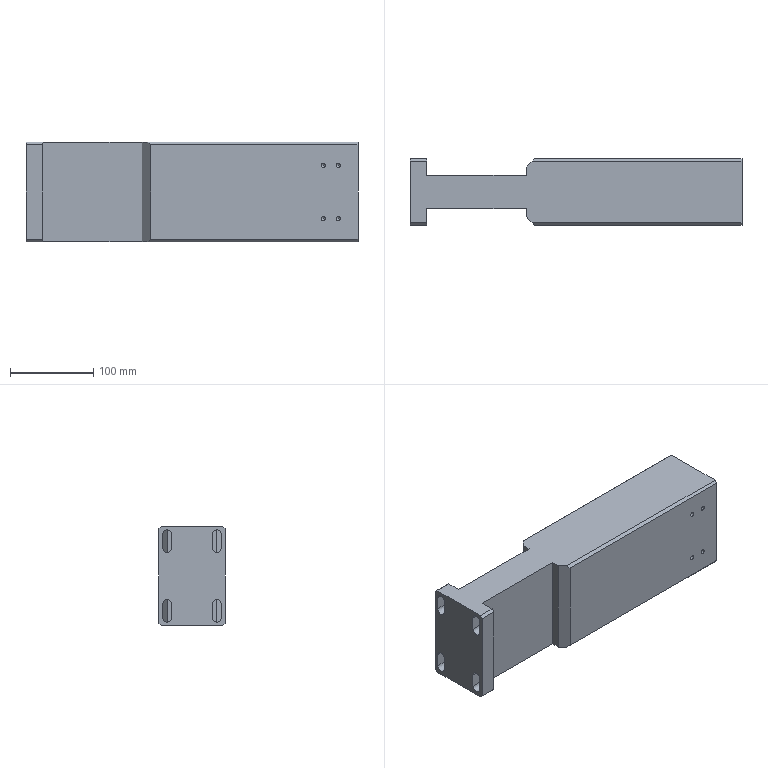CAM job | NX | 3+2 milling, drilling | part box 400 x 80 x 120 mm | stock box 405 x 85 x 125 mm
Tools:
number,name,description,diameter,corner_radius,flute_length,length,flutes
9,D10,平底铣刀-粗,10.0,0.0,35.0,75.0,2
17,D16,平底铣刀-粗,16.0,0.0,50.0,75.0,2
10,D10-J,平底铣刀-精,10.0,0.0,35.0,75.0,2
18,D16-J,平底铣刀-精,16.0,0.0,50.0,75.0,2
19,D6R0.5,圆鼻刀-粗,6.0,0.5,50.0,75.0,2
1,D80R0.8飞刀,圆鼻刀-粗,80.0,0.8,50.0,75.0,2
1,D80R0.8飞刀-J,圆鼻刀-精,80.0,0.8,50.0,75.0,2
2,D6倒角刀,倒角刀,6.0,0.0,3.0,25.0,2
20,D10倒角刀,倒角刀,10.0,0.0,5.0,75.0,2
23,M6X1.0,丝锥,5.0,0.0,35.0,50.0,2
15,ZT5,钻头,5.0,0.0,35.0,50.0,2
Operations:
program,operation,operation_type,tool,method,geometry_group,spindle_rpm,surface_speed,feed_per_tooth,feed_cut,feed_plunge,cut_length_mm,path_length_mm,cut_time_min,machine_time_min
B,底壁铣飞面开粗_COPY,VolumeBased25DMillingOperation,D80R0.8飞刀,分层开粗-切深K-步距G,W-B,5000.0,1256.637,0.3,3000.0,100.0,9417.187,9967.757,3.139,3.194
B,底壁铣飞面精光_COPY,VolumeBased25DMillingOperation,D80R0.8飞刀-J,侧刃精光-切深K-步距G,W-B,5000.0,1256.637,0.1,1000.0,100.0,1045.766,1081.766,1.046,1.049
B,型腔铣开粗-中_COPY_COPY,CavityMilling,D10,分层开粗-切深K-步距G,W-B,8000.0,251.327,0.375,6000.0,100.0,58997.485,61169.673,9.833,10.153
B,打点-深0.8_2,Operation,D6倒角刀,NONE,W-B,8000.0,150.796,0.0312,500.0,90.0,7.2,157.463,0.0144,0.0294
B,盲锥孔-M6螺纹底孔_2,Operation,ZT5,NONE,W-B,2500.0,39.27,0.06,300.0,90.0,78.009,299.08,0.26,0.2821
B,等高精光往复爬面_COPY_COPY,ZLevelMilling,D6R0.5,等高爬面-切深K-步距G,W-B,7000.0,131.947,0.3571,5000.0,100.0,15071.804,15111.489,3.014,3.018
B,平面去毛刺6X45L_COPY,SurfaceContour,D6倒角刀,爬面_倒角-切深0-步距G,W-B,6500.0,122.519,0.1154,1500.0,100.0,692.088,1885.62,0.4614,0.5807
B,铣倒角_2,PlanarMilling,D6倒角刀,METHOD,W-B,8000.0,150.796,0.0375,600.0,100.0,75.821,342.245,0.1264,0.153
B,底壁铣倒角_COPY_COPY,VolumeBased25DMillingOperation,D10倒角刀,爬面_倒角-切深0-步距G,W-B,6500.0,122.519,0.1154,1500.0,100.0,608.074,1144.494,0.4054,0.459
B,盲锥孔-攻牙M6_2,Operation,M6X1.0,METHOD,W-B,500.0,7.854,0.001,1.0,90.0,64.0,271.063,64.0,64.021
B,底壁铣精光底面-中_COPY_1,VolumeBased25DMillingOperation,D10-J,精光步距切深关,W-B,8000.0,251.32,0.0625,1000.0,100.0,3094.541,3161.141,3.095,3.101
B,底壁铣精光侧面-中-选底面_COPY_1,VolumeBased25DMillingOperation,D10-J,侧刃精光-切深K-步距G,W-B,8000.0,251.32,0.0625,1000.0,100.0,277.362,450.564,0.2774,0.2947
A,顶面,FaceMilling,D80R0.8飞刀,侧刃精光-切深K-步距G,W-A,5000.0,1256.637,0.1,1000.0,100.0,1040.667,1076.667,1.041,1.044
A,外形粗_2,VolumeBased25DMillingOperation,D16,METHOD,W-A,5000.0,251.327,0.5,5000.0,80.0,89454.829,89573.829,17.891,17.903
A,型腔铣开粗-中_COPY,CavityMilling,D10,分层开粗-切深K-步距G,W-A,8000.0,251.327,0.375,6000.0,100.0,81391.286,84732.281,13.565,14.04
A,打点-深0.8,Operation,D6倒角刀,NONE,W-A,8000.0,150.796,0.0312,500.0,90.0,7.2,157.463,0.0144,0.0294
A,盲锥孔-M6螺纹底孔,Operation,ZT5,NONE,W-A,2500.0,39.27,0.06,300.0,90.0,78.009,299.08,0.26,0.2821
A,等高精光往复爬面_COPY,ZLevelMilling,D6R0.5,等高爬面-切深K-步距G,W-A,7000.0,131.947,0.3571,5000.0,100.0,15071.803,15103.463,3.014,3.018
A,铣倒角_1,PlanarMilling,D6倒角刀,METHOD,W-A,8000.0,150.796,0.0375,600.0,100.0,75.821,342.245,0.1264,0.153
A,仅选体,SurfaceContour,D6倒角刀,METHOD,W-A,8000.0,150.796,0.1875,3000.0,100.0,673.495,1678.556,0.2245,0.325
A,底壁铣倒角_COPY,VolumeBased25DMillingOperation,D10倒角刀,爬面_倒角-切深0-步距G,W-A,6500.0,122.519,0.1154,1500.0,100.0,608.074,1144.494,0.4054,0.459
A,盲锥孔-攻牙M6,Operation,M6X1.0,METHOD,W-A,500.0,7.854,0.001,1.0,90.0,64.0,271.063,64.0,64.021
A,底壁铣精光底面-中_COPY,VolumeBased25DMillingOperation,D10-J,精光步距切深关,W-A,8000.0,251.32,0.0625,1000.0,100.0,3094.541,3152.341,3.095,3.1
A,底壁铣精光侧面-中-选底面_COPY,VolumeBased25DMillingOperation,D10-J,侧刃精光-切深K-步距G,W-A,8000.0,251.32,0.0625,1000.0,100.0,554.724,920.403,0.5547,0.5913
A,外形半精_2,VolumeBased25DMillingOperation,D16-J,METHOD,W-A,5000.0,251.327,0.1,1000.0,100.0,5476.257,6164.298,5.476,5.545